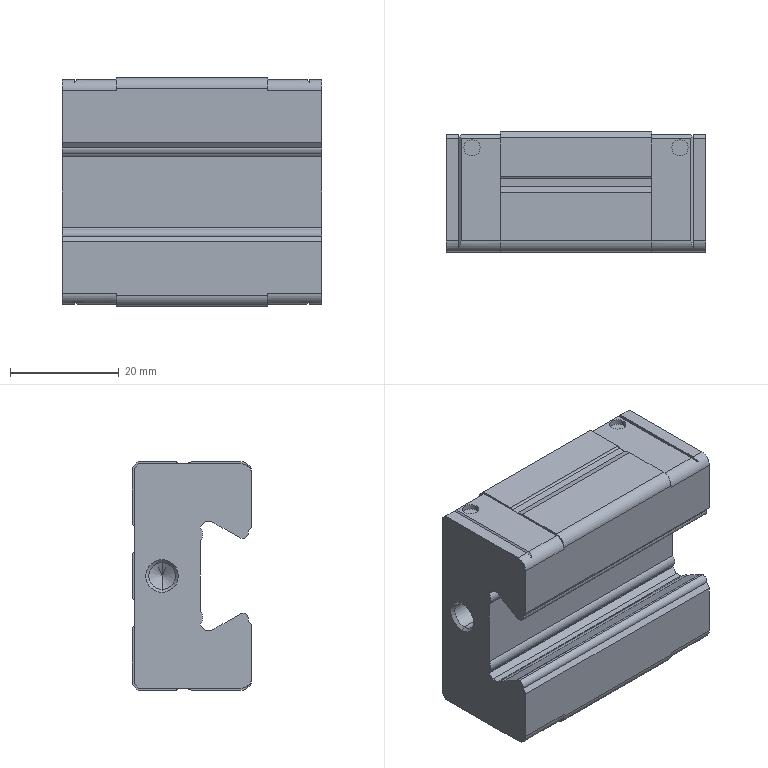Part | STEP file | SSR20XVUUB Slide15-25 | 1 solid | 127 faces | box 47.7 x 22 x 42 mm | volume 34844 mm3 | plane 78 | cylinder 33 | cone 16 | commonest cylinder face diameters 3 x8 4 x6 3.3 x4 4.134 x4 4.917 x4 2 x3